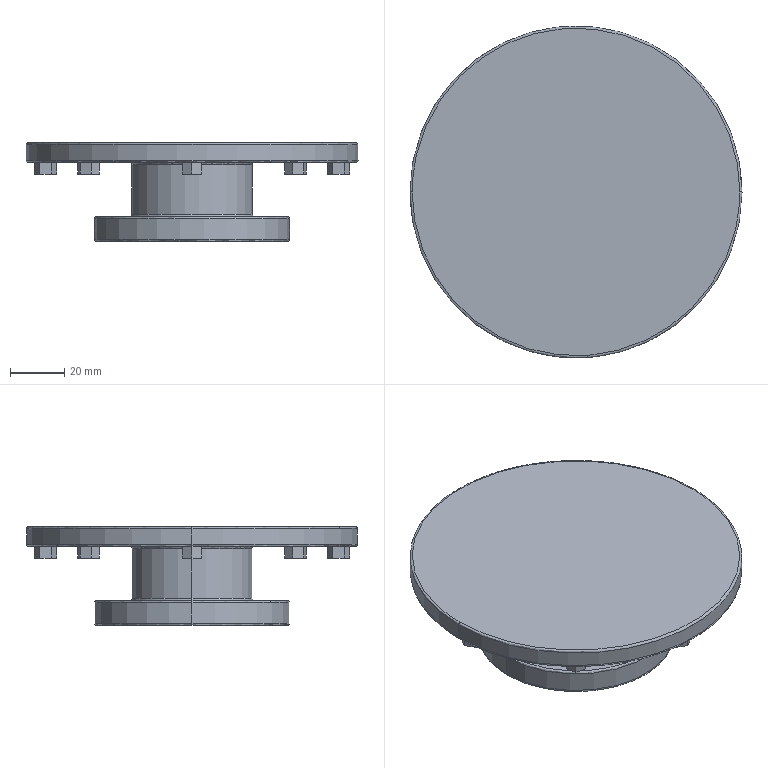Part | STEP file | XB-Connecting flange_BWED3922_90B5.step | 1 solid | 101 faces | box 122.4 x 122.4 x 36.36 mm | volume 150900 mm3 | plane 66 | cylinder 18 | spline 16 | cone 1 | commonest cylinder face diameters 4.32 x8 8.64 x2 44.46 x2 46.8 x2 72 x2 122.4 x2